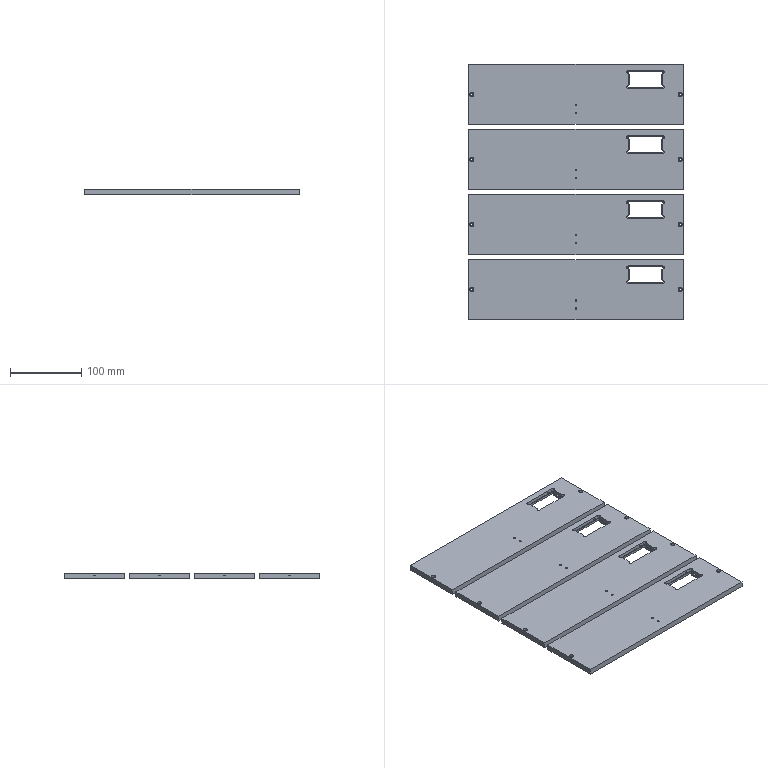CAM job | NX | 3-axis milling | part box 300 x 357 x 8 mm | stock box 306 x 363 x 8 mm
Tools:
number,name,description,diameter,corner_radius,flute_length,length,flutes
2,D4A45,Milling Tool-5 Parameters,4.0,0.0,2.0,2.0,2
6,D6,Milling Tool-5 Parameters,6.0,0.0,50.0,75.0,2
4,D4,Milling Tool-5 Parameters,4.0,0.0,50.0,75.0,2
12,D2,Milling Tool-5 Parameters,2.0,0.0,50.0,75.0,2
15,D1.5,Milling Tool-5 Parameters,1.5,0.0,50.0,75.0,2
Operations:
program,operation,operation_type,tool,method,geometry_group,spindle_rpm,surface_speed,feed_per_tooth,feed_cut,feed_plunge,cut_length_mm,path_length_mm,cut_time_min,machine_time_min
1吸,ZLEVEL_PROFILE_1_COPY_1_COPY_COPY,ZLevelMilling,D4A45,METHOD,A,9500.0,179.0,0.0526,1000.0,100.0,3909.557,8466.182,3.91,4.365
1吸,ZLEVEL_PROFILE_COPY_COPY_1_COPY,ZLevelMilling,D6,METHOD,A,9500.0,179.0,0.1158,2200.0,1000.0,50666.545,51330.931,23.113,23.179
1吸,ZLEVEL_PROFILE_COPY_COPY_1_COPY_COPY_COPY,ZLevelMilling,D6,METHOD,A,9500.0,179.0,0.0868,1650.0,1000.0,7506.034,8085.523,4.609,4.667
1吸,ZLEVEL_PROFILE_COPY_COPY_1_COPY_COPY,ZLevelMilling,D6,METHOD,A,9500.0,179.0,0.0868,1650.0,1000.0,5232.334,5807.573,3.231,3.289
1吸,HOLE_MILLING_COPY,CylinderMilling,D4,METHOD,A,9500.0,179.0,0.0789,1500.0,100.0,579.071,1921.071,0.386,0.5202
1吸,ZLEVEL_PROFILE_COPY_COPY_1_COPY_COPY_COPY_1,ZLevelMilling,D4,METHOD,A,9500.0,179.0,0.0868,1650.0,1000.0,1983.24,5294.888,1.31,1.642
1吸,HOLE_MILLING_COPY_COPY,CylinderMilling,D2,METHOD,A,9500.0,59.0,0.0526,1000.0,100.0,1276.104,2680.904,1.276,1.417
1吸,HOLE_MILLING_COPY_COPY_1,CylinderMilling,D1.5,METHOD,A,9500.0,44.0,0.0368,700.0,100.0,1438.349,2261.349,2.055,2.137
1吸,ZLEVEL_PROFILE_COPY_COPY_COPY_COPY_COPY,ZLevelMilling,D4,MILL_FINISH,A,9500.0,119.0,0.0632,1200.0,1000.0,3138.39,4586.758,2.617,2.761